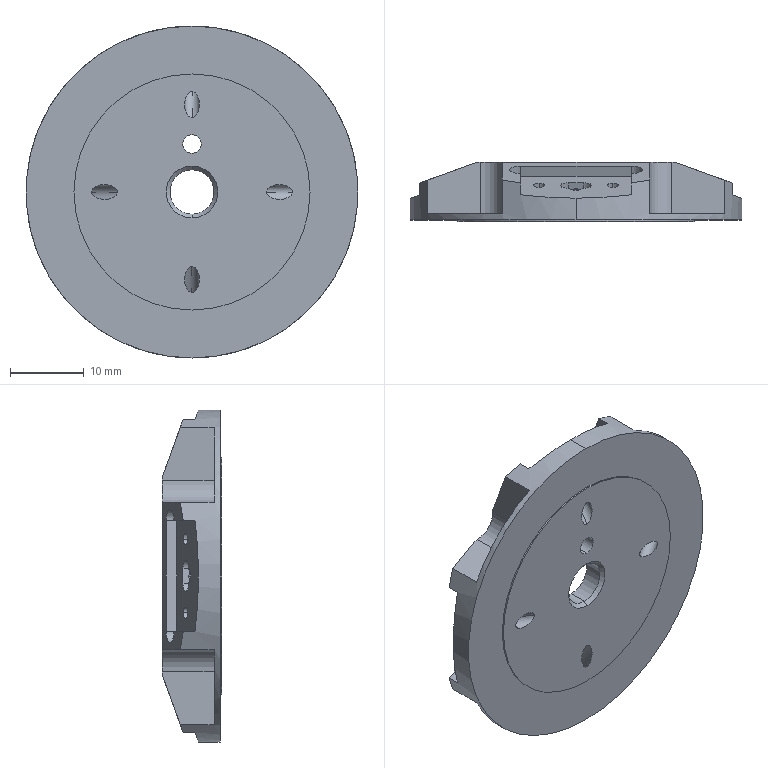Part | SolidWorks | features ICE 14, CirPattern 5, Chamfer 2, Extrusion 1, Fillet 1, HoleWzd 1 | 1 solid | 133 faces | box 45 x 8 x 45 mm | volume 6154 mm3 | plane 59 | cylinder 54 | cone 20 | commonest cylinder face diameters 1.6 x16 2 x8 2.2 x8 3 x8 6 x6 2.5 x2